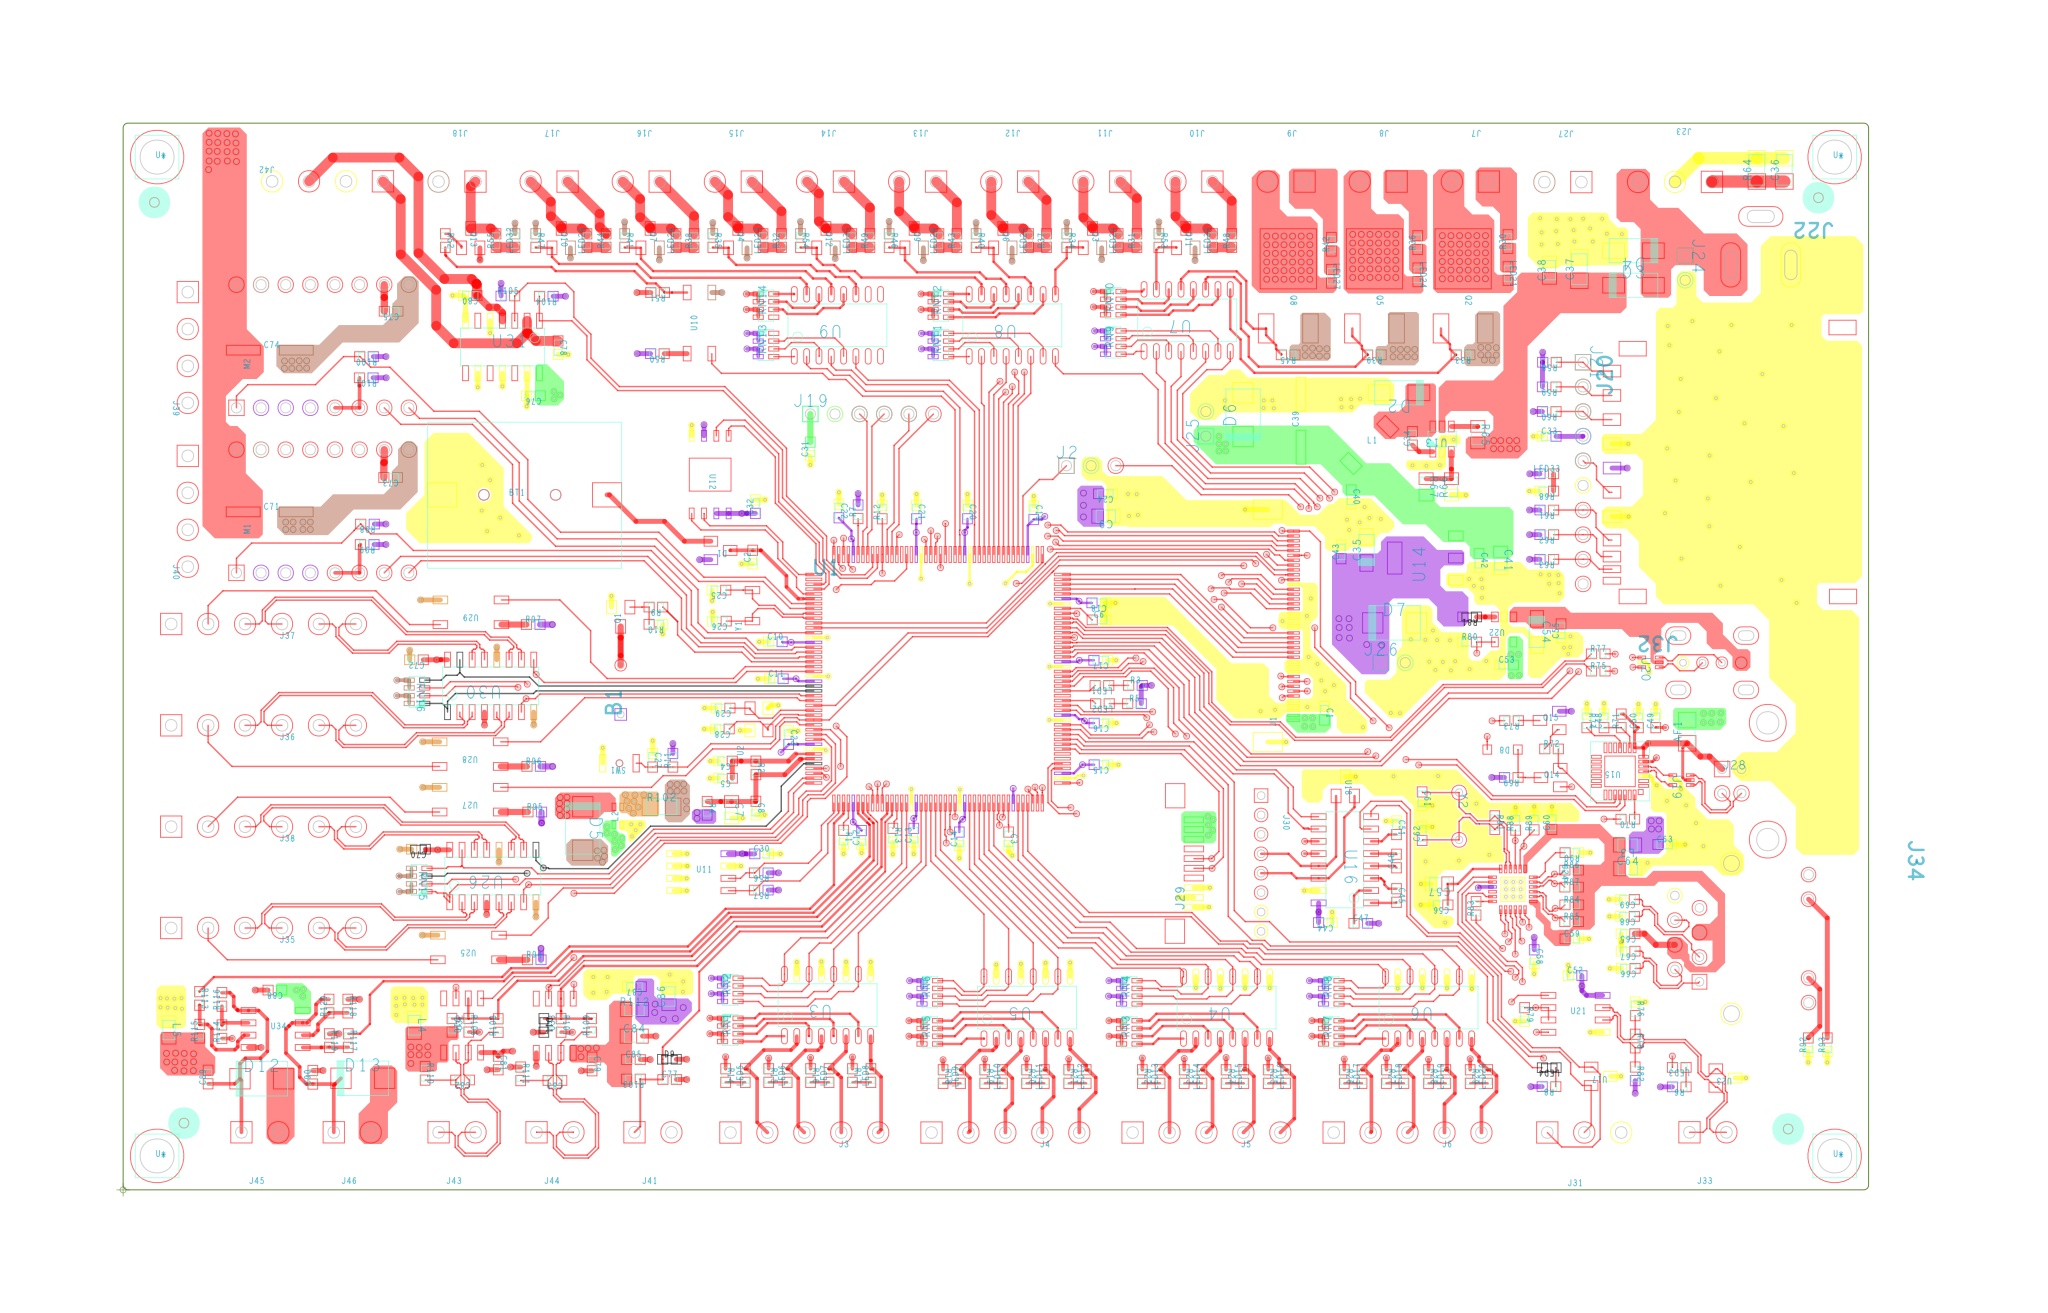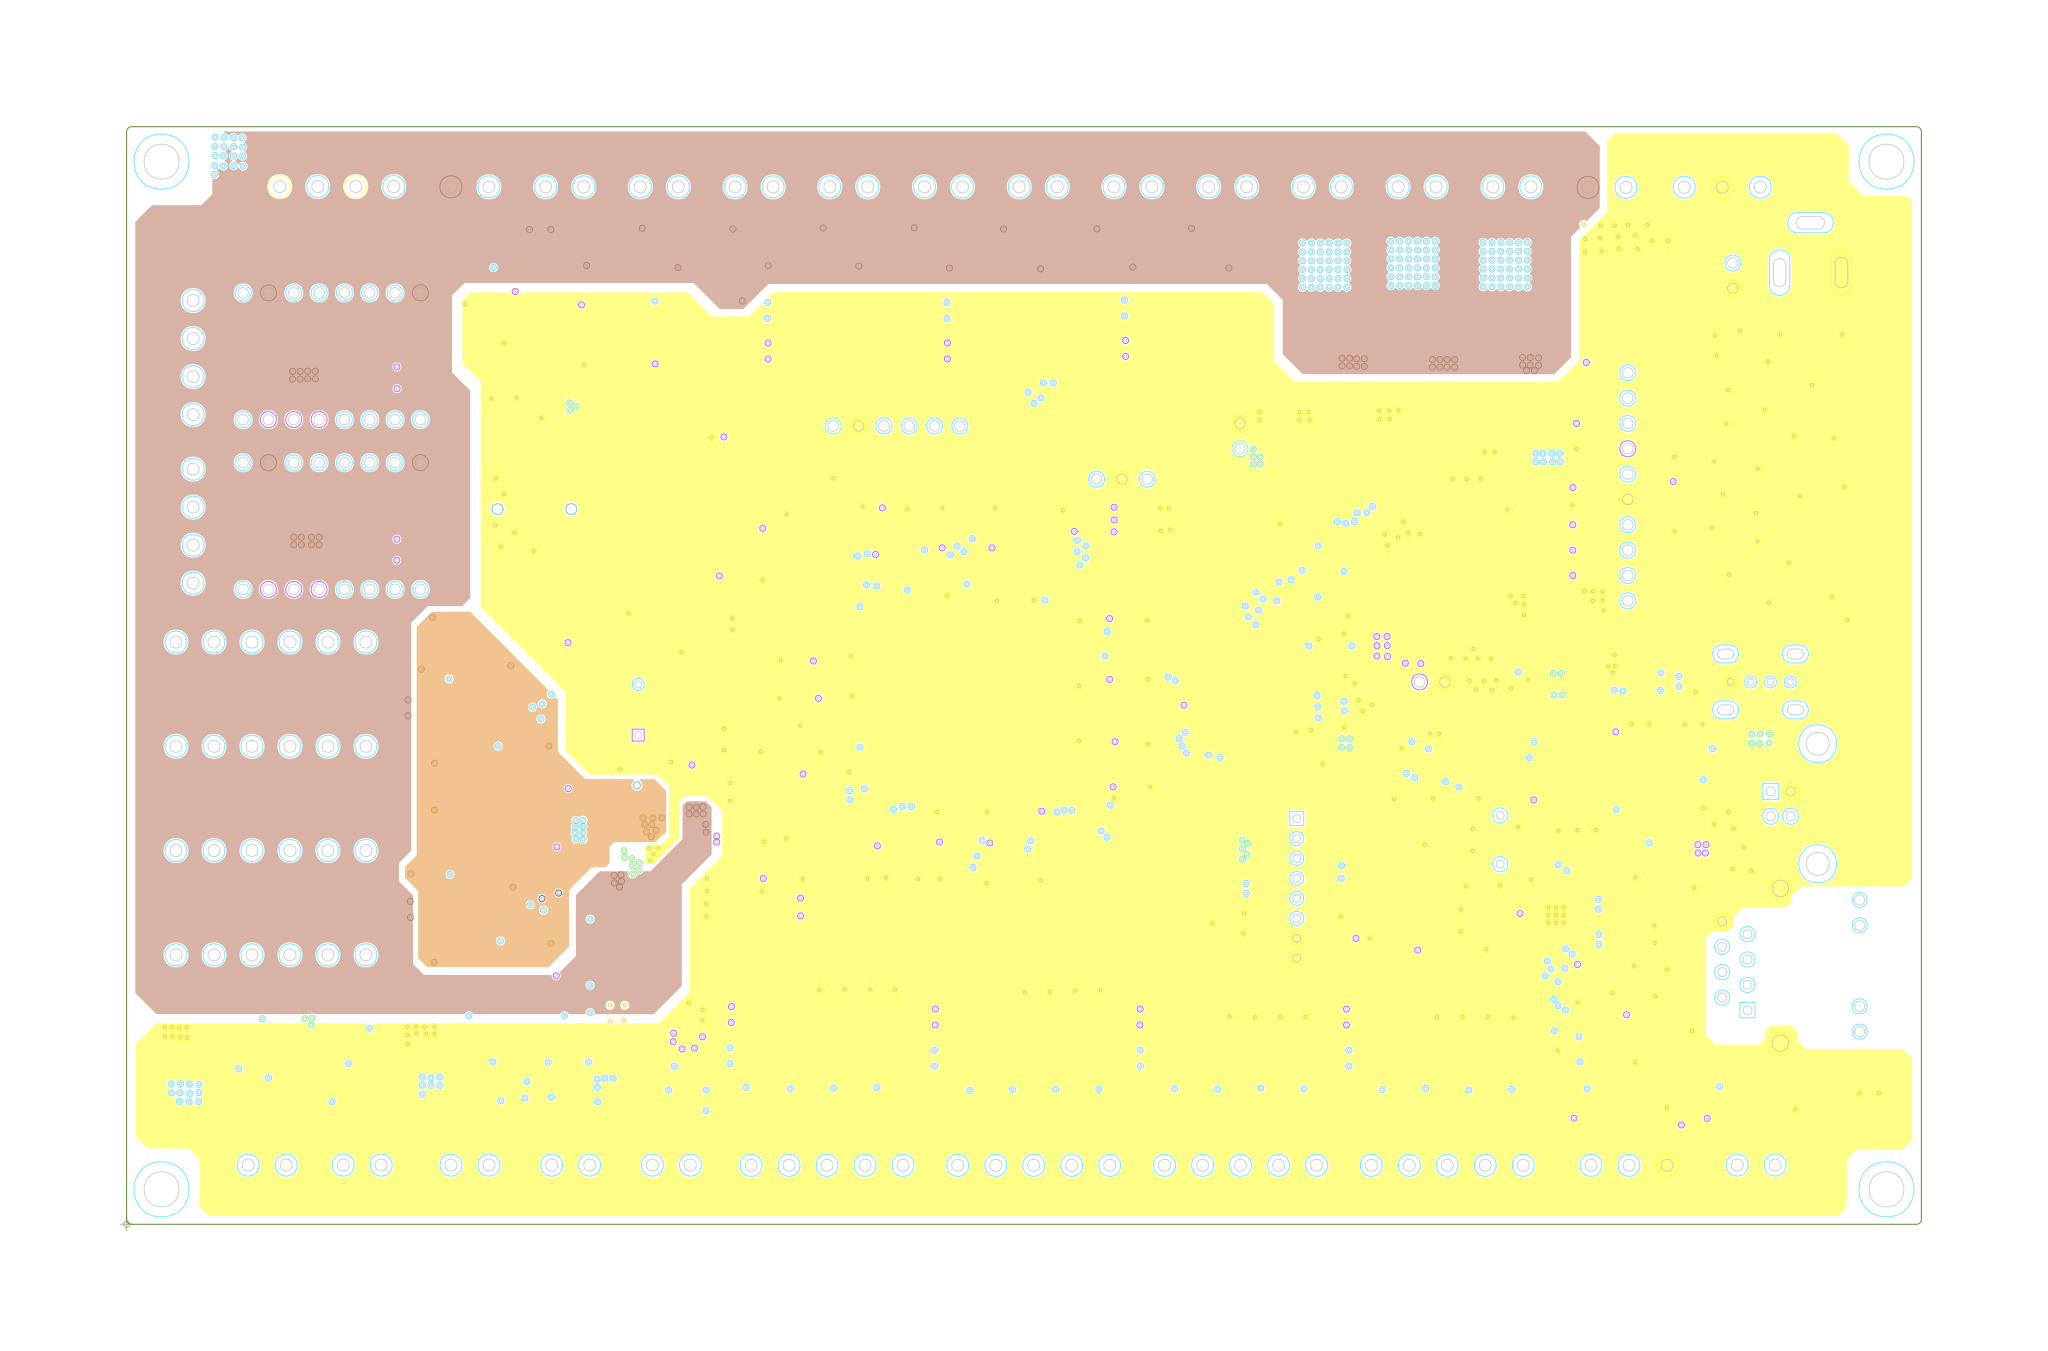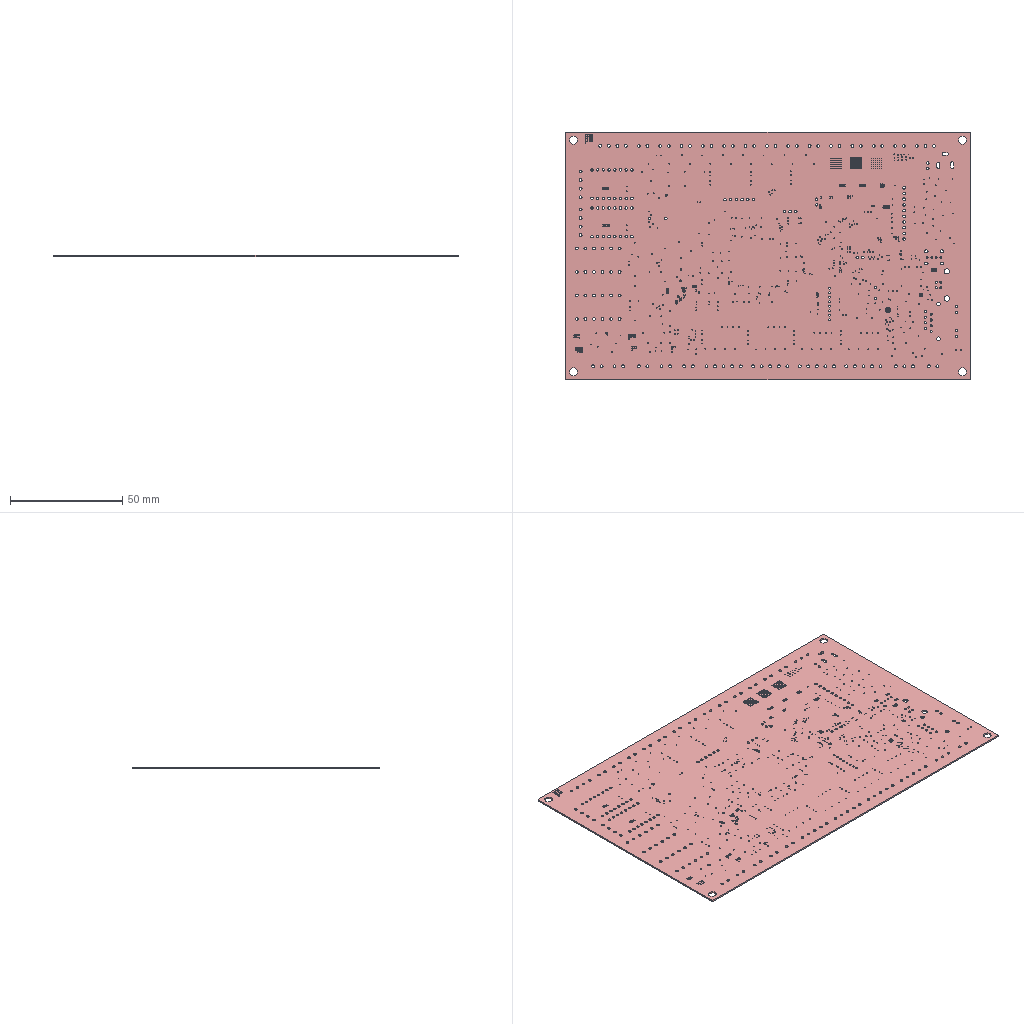Circuit board layout | Cadence Allegro | box 180 x 110 x 0.7 mm
Layer stack:
# Cadence Allegro layer stack of  (unit mm; from the constraint file cross-section; dielectric type: 0 not recorded (Allegro does not mark core vs prepreg), 3 surface material)
index,name,kind,layer,copper_thickness_mm,dielectric_type,dielectric_thickness_mm,dielectric_material,dielectric_constant
0,Top Surface,other,,,,,,
1,TOP,copper,TOP,0.0305,,,,
2,Dielectric1,dielectric,,,0,0.2032,FR-4,4.5
3,GND02,copper,GND02,0.0305,,,,
4,Dielectric2,dielectric,,,0,0.2032,FR-4,4.5
5,PWR03,copper,PWR03,0.0305,,,,
6,Dielectric3,dielectric,,,0,0.2032,FR-4,4.5
7,BOTTOM,copper,BOTTOM,0.0305,,,,
8,Bottom Surface,other,,,,,,
# drill layer pairs: low layer,high layer
drill_pair,TOP,BOTTOM
Part placement:
REFDES,COMP_VALUE,SYM_NAME,SYM_X,SYM_Y,SYM_ROTATE,SYM_MIRROR
AF1,500mA,R1206,6350.000,1860.000,90.000,NO
B1,BEEP,BELL-5,2020.000,1930.000,90.000,NO
BT1,BATTERY,BATSO,2004.016,2821.579,0.000,NO
C1,0.1uF,C0603,4877.402,1935.000,270.000,NO
C2,0.1uF,C0603,2556.000,2569.000,90.000,NO
C3,2.2uF,C0603,3595.000,1425.000,270.000,NO
C4,0.1uF,C0603,2445.701,1741.000,180.000,NO
C5,2.2uF,C0603,2445.701,1671.000,180.000,NO
C6,2.2uF,C0603,3962.000,2314.000,0.000,NO
C7,10uF,C0805,2470.000,1543.000,270.000,NO
C8,0.1uF,C0603,2569.000,1550.000,270.000,NO
C9,10uF,C0805,3990.000,2735.000,180.000,NO
C10,0.1uF,C0603,2648.000,2225.000,0.000,NO
C11,0.1uF,C0603,2652.000,2075.000,0.000,NO
C12,0.1uF,C0603,2998.000,1431.000,90.000,NO
C13,0.1uF,C0603,3210.000,1440.000,90.000,NO
C14,0.1uF,C0603,3395.000,1425.000,90.000,NO
C15,0.1uF,C0603,3970.000,1726.000,180.000,NO
C16,0.1uF,C0603,3970.000,1895.000,180.000,NO
C17,0.1uF,C0603,3969.000,2150.000,180.000,NO
C18,0.1uF,C0603,3961.000,2383.000,180.000,NO
C19,0.1uF,C0603,3697.000,2749.000,270.000,NO
C20,0.1uF,C0603,3428.000,2752.000,270.000,NO
C21,0.1uF,C0603,3221.000,2752.000,270.000,NO
C22,0.1uF,C0603,2906.000,2756.000,270.000,NO
C23,0.1uF,C0603,2702.000,1836.000,270.000,NO
C24,0.1uF,C0603,3988.000,2826.000,180.000,NO
C25,6pF,C0603,2419.000,2435.000,180.000,NO
C26,6pF,C0603,2421.000,2309.000,180.000,NO
C27,0.1uF,C0603,2150.000,1744.000,270.000,NO
C28,22pF,C0603,2433.000,1871.000,180.000,NO
C29,22pF,C0603,2436.000,1956.000,180.000,NO
C30,0.1uF,C0603,2592.000,1364.000,0.000,NO
C31,0.1uF,C0603,2790.000,3008.000,90.000,NO
C32,0.1uF,C0603,2567.000,2774.000,90.000,NO
C33,0.1uF,C0603,5790.000,3059.000,0.000,NO
C34,0.01uF,C0603,5235.000,3051.000,90.000,NO
C35,10V/10uF,TA3216,5048.000,2598.000,90.000,NO
C36,1nF/250V,C1206,6745.000,4141.000,90.000,NO
C37,10uF 50V,C1206,5912.406,3738.000,90.000,NO
C38,0.1uF 50V,C0805,5791.000,3734.000,90.000,NO
C39,16V/220uF,SMD-EC-6_3,4782.000,3015.000,90.000,NO
C40,0.1uF,C0603,4986.000,2814.000,270.000,NO
C41,10uF,C0805,5593.000,2556.000,270.000,NO
C42,0.1uF,C0603,5505.000,2556.000,270.000,NO
C43,0.1uF,C0603,4945.000,2590.000,90.000,NO
C44,0.1uF,C0603,4881.000,1085.000,180.000,NO
C45,0.1uF,C0603,5170.000,1195.000,270.000,NO
C46,0.1uF,C0603,5170.000,1335.000,90.000,NO
C47,0.1uF,C0603,5025.000,1082.000,0.000,NO
C48,0.1uF,C0603,6012.402,1904.055,90.000,NO
C49,0.1uF,C0603,6222.406,1904.055,90.000,NO
C50,0.1uF,C0603,6152.402,1904.055,90.000,NO
C51,0.1uF,C0603,5170.000,1470.000,270.000,NO
C52,0.1uF,C0603,5895.000,870.000,0.000,NO
C53,0.1uF,C0603,5617.000,2131.000,0.000,NO
C54,22uF,TA3216,5740.000,2265.000,270.000,NO
C55,0.1uF,C0603,5838.000,2270.000,90.000,NO
C56,0.1uF,C0603,5351.000,1157.000,180.000,NO
C57,10uF,C0805,5344.000,1242.000,180.000,NO
C58,0.1uF,C0603,5729.000,947.000,270.000,NO
C59,0.1uF,C0603,5882.000,1019.000,0.000,NO
C60,0.1uF,C0603,5801.000,1491.000,90.000,NO
C61,22pF,C0603,5274.000,1588.000,270.000,NO
C62,22pF,C0603,5274.000,1446.000,90.000,NO
C63,0.1uF,C0603,6259.000,1402.000,0.000,NO
C64,10uF,C0805,6109.000,1304.000,0.000,NO
C65,22nF,C0603,6110.000,1040.000,180.000,NO
C66,10pF,C0603,6111.000,899.000,180.000,NO
C67,10pF,C0603,6110.402,969.000,180.000,NO
C68,10pF,C0603,6108.000,1110.000,180.000,NO
C69,10pF,C0603,6108.000,1179.000,180.000,NO
C70,0.1uF,C0603,1199.000,1383.000,180.000,NO
C71,100uF 35V,SMD-EC-6_3,487.500,2752.500,0.000,NO
C72,0.1uF,C0603,1191.000,2152.000,180.000,NO
C73,0.1uF,C0603,1086.000,2892.000,180.000,NO
C74,100uF 35V,SMD-EC-6_3,488.000,3409.000,0.000,NO
C75,0.1uF,C0603,1088.000,3567.000,180.000,NO
C76,0.1uF,C0603,1666.000,3224.000,180.000,NO
C77,0.1uF,C0603,2219.000,448.000,0.000,NO
C78,0.1uF,C0603,1766.000,3419.000,270.000,NO
C79,0.1uF,C0603,1904.000,511.000,270.000,NO
C80,0.1uF,C0603,1409.000,3631.000,180.000,NO
C81,0.1uF,C0603,1523.000,515.000,270.000,NO
C82,0.1uF,C0603,1378.000,446.000,180.000,NO
C83,0.1uF,C0603,1753.000,444.000,180.000,NO
C84,10uF,C0805,2075.000,624.000,0.000,NO
C85,0.1uF,C0603,2072.000,529.000,0.000,NO
C86,10uF,C0805,2216.000,785.000,90.000,NO
C87,0.1uF,C0603,2076.000,825.000,180.000,NO
C88,0.1uF,C0603,616.000,811.000,180.000,NO
C89,0.1uF,C0603,345.000,458.000,90.000,NO
C90,0.1uF,C0603,770.000,457.000,90.000,NO
D1,BAT54C,SOT-23,2425.000,2596.000,180.000,NO
D2,SS14,DO-214AC,5180.000,3236.000,180.000,NO
D3,SS14,DO-214AC,6132.110,3672.409,0.000,NO
D4,SS14,DO-214AC,6132.000,3813.000,180.000,NO
D5,SMBJ5.0A,DO-214AA,1866.000,1467.000,270.000,NO
D6,SMBJ5.0A,DO-214AA,4547.000,3147.000,90.000,NO
D7,SMBJ3.3A,DO-214AA,5162.000,2301.803,0.000,NO
D8,1N4148,SOD123,5662.445,1787.402,180.000,NO
D9,CG0603MLC,R0603,2218.000,530.000,0.000,NO
D10,CG0603MLC,R0603,1335.071,668.051,270.000,NO
D11,CG0603MLC,R0603,1708.000,667.433,270.000,NO
D12,SMBJ10CA,DO-214AA,563.000,451.000,0.000,NO
D13,SMBJ10CA,DO-214AA,973.000,453.000,0.000,NO
J1,RGBLCD,FPC-TOP40,4755.890,1906.642,90.000,NO
J2,SWD,CON2_54X1X3,3830.000,2940.000,0.000,NO
J3,HEADER 5,SIP3_81X1X5,2465.591,232.638,0.000,NO
J4,HEADER 5,SIP3_81X1X5,3281.969,232.638,0.000,NO
J5,HEADER 5,SIP3_81X1X5,4098.346,232.638,0.000,NO
J6,HEADER 5,SIP3_81X1X5,4914.724,232.638,0.000,NO
J7,HEADER 2,SIP3_81X1X2,5544.626,4093.402,180.000,NO
J8,HEADER 2,SIP3_81X1X2,5170.610,4093.402,180.000,NO
J9,HEADER 2,SIP3_81X1X2,4796.594,4093.402,180.000,NO
J10,HEADER 2,SIP3_81X1X2,4422.579,4093.402,180.000,NO
J11,HEADER 2,SIP3_81X1X2,4048.563,4093.402,180.000,NO
J12,HEADER 2,SIP3_81X1X2,3674.547,4093.402,180.000,NO
J13,HEADER 2,SIP3_81X1X2,3300.531,4093.402,180.000,NO
J14,HEADER 2,SIP3_81X1X2,2926.516,4093.402,180.000,NO
J15,HEADER 2,SIP3_81X1X2,2552.500,4093.402,180.000,NO
J16,HEADER 2,SIP3_81X1X2,2178.484,4093.402,180.000,NO
J17,HEADER 2,SIP3_81X1X2,1804.469,4093.402,180.000,NO
J18,HEADER 2,SIP3_81X1X2,1430.453,4093.402,180.000,NO
J19,ATK MODULE,CON2_54X1X6,2790.000,3150.000,0.000,NO
J20,SD_CARD_L,SDCARD_L,6044.500,3225.000,90.000,NO
J21,SD,CON2_54X1X10,5927.402,3360.000,270.000,NO
J22,DC_SOCKET,DC10B,6946.000,3925.130,180.000,NO
J23,SIP3-3.81,SIP3_81X1X3,6450.551,4092.165,180.000,NO
J24,TEST24V,CON2_54X1X2,6342.000,3793.000,270.000,NO
J25,TEST5V,CON2_54X1X2,4396.000,3060.000,90.000,NO
J26,TEST3.3V,CON2_54X1X2,5105.469,2140.000,0.000,NO
J27,HEADER 2,SIP3_81X1X2,5920.354,4091.378,180.000,NO
J28,USB_TYPEB,USB-B-90,6491.846,1708.260,0.000,NO
J29,TTL_LCD,FFC-1_0-10P,4307.827,1136.035,90.000,NO
J30,UART_LCD,CI0608,4620.157,1600.591,270.000,NO
J31,RS232,SIP3_81X1X3,5782.126,232.835,0.000,NO
J32,USB-A-90,USB-A-90,6313.701,2246.303,180.000,NO
J33,HEADER 2,SIP3_81X1X2,6359.370,233.622,0.000,NO
J34,RJ45,HR911105A,6650.000,1020.004,270.000,NO
J35,X  AXIS,SIP3_81X1X6,195.000,1063.071,0.000,NO
J36,Z  AXIS,SIP3_81X1X6,195.000,1885.906,0.000,NO
J37,A  AXIS,SIP3_81X1X6,195.000,2297.323,0.000,NO
J38,Y AXIS,SIP3_81X1X6,195.000,1474.488,0.000,NO
J39,C  AXIS,SIP3_81X1X4,262.441,3644.803,270.000,NO
J40,B  AXIS,SIP3_81X1X4,262.441,2979.803,270.000,NO
J41,HEADER 2,SIP3_81X1X2,2076.063,233.622,0.000,NO
J42,HEADER 4,SIP3_81X1X4,1054.803,4094.583,180.000,NO
J43,HEADER 2,SIP3_81X1X2,1280.787,233.622,0.000,NO
J44,HEADER 2,SIP3_81X1X2,1678.425,233.622,0.000,NO
J45,HEADER 2,SIP3_81X1X2,480.197,233.622,0.000,NO
J46,HEADER 2,SIP3_81X1X2,855.197,233.622,0.000,NO
L1,4.7uH,SMD-L5_1W5_1_H3_0,5060.000,3024.000,0.000,NO
L2,ACM2012,ACM2012,1993.000,1482.000,90.000,NO
L3,220R,2A,0.05DCR,R0805,6108.000,1400.000,180.000,NO
L4,330OHM,R0805,1182.000,668.000,270.000,NO
L5,330OHM,R0805,186.000,649.000,270.000,NO
LED1,LED,LED0603,3974.000,2048.000,180.000,NO
LED2,LED,LED0603,3976.000,1974.000,180.000,NO
LED3,LED,LED0603,6318.000,497.000,180.000,NO
LED4,LED,LED0603,5790.000,496.000,180.000,NO
LED5,LED,LED0603,2526.000,464.000,90.000,NO
LED6,LED,LED0603,2696.000,464.000,90.000,NO
LED7,LED,LED0603,2866.000,464.000,90.000,NO
LED8,LED,LED0603,3036.000,464.000,90.000,NO
LED9,LED,LED0603,3400.000,460.000,90.000,NO
LED10,LED,LED0603,3570.000,460.000,90.000,NO
LED11,LED,LED0603,3740.000,460.000,90.000,NO
LED12,LED,LED0603,3910.000,460.000,90.000,NO
LED13,LED,LED0603,4210.000,460.000,90.000,NO
LED14,LED,LED0603,4380.000,460.000,90.000,NO
LED15,LED,LED0603,4550.000,460.000,90.000,NO
LED16,LED,LED0603,4720.000,460.000,90.000,NO
LED17,LED,LED0603,5030.000,460.000,90.000,NO
LED18,LED,LED0603,5200.000,460.000,90.000,NO
LED19,LED,LED0603,5370.000,460.000,90.000,NO
LED20,LED,LED0603,5540.000,460.000,90.000,NO
LED21,LED,LED0603,5622.551,3720.000,270.000,NO
LED22,LED,LED0603,4040.055,3854.000,90.000,NO
LED23,LED,LED0603,2598.055,3854.000,90.000,NO
LED24,LED,LED0603,5256.551,3715.000,270.000,NO
LED25,LED,LED0603,3676.055,3854.000,90.000,NO
LED26,LED,LED0603,2245.055,3854.000,90.000,NO
LED27,LED,LED0603,4905.551,3709.000,270.000,NO
LED28,LED,LED0603,3312.055,3854.000,90.000,NO
LED29,LED,LED0603,1883.055,3854.000,90.000,NO
LED30,LED,LED0603,4423.000,3854.000,90.000,NO
LED31,LED,LED0603,2958.055,3854.000,90.000,NO
LED32,LED,LED0603,1591.000,3854.000,90.000,NO
LED33,LED,LED0603,5780.000,2907.000,0.000,NO
M1,STEPSTICK,STEPSTICK,460.000,2505.000,90.000,NO
M2,STEPSTICK,STEPSTICK,460.000,3175.000,90.000,NO
Q1,8050,SOT-23,2020.000,2327.000,90.000,NO
Q2,FR540,TO-252AA,5440.551,3780.000,270.000,NO
Q3,PMV60EN,SOT-23,3935.528,3863.500,270.000,NO
Q4,PMV60EN,SOT-23,2495.528,3863.500,270.000,NO
Q5,FR540,TO-252AA,5080.551,3780.000,270.000,NO
Q6,PMV60EN,SOT-23,3571.528,3863.500,270.000,NO
Q7,PMV60EN,SOT-23,2139.528,3863.500,270.000,NO
Q8,FR540,TO-252AA,4730.551,3780.000,270.000,NO
Q9,PMV60EN,SOT-23,3211.528,3863.500,270.000,NO
Q10,PMV60EN,SOT-23,1778.528,3863.500,270.000,NO
Q11,PMV60EN,SOT-23,4314.528,3863.500,270.000,NO
Q12,PMV60EN,SOT-23,2853.528,3863.500,270.000,NO
Q13,PMV50EP,SOT-23,1411.000,3863.500,270.000,NO
Q14,S8050,SOT-23,5795.902,1673.555,0.000,NO
Q15,S8550,SOT-23,5791.902,1905.555,0.000,NO
R1,10K,R0603,2925.000,1432.000,270.000,NO
R2,10R,R0603,2569.000,1713.000,270.000,NO
R3,510R,R0603,4110.000,2048.000,0.000,NO
R4,10R,R0603,2371.000,1549.000,270.000,NO
R5,510R,R0603,4106.000,1974.000,0.000,NO
R6,510R,R0603,6318.000,418.000,180.000,NO
R7,0R,R0603,2984.000,2753.000,90.000,NO
R8,510R,R0603,5789.000,419.000,180.000,NO
R9,510R,R0603,2163.000,2366.000,180.000,NO
R10,10K,R0603,2163.000,2296.000,180.000,NO
R11,10K,R0603,2232.000,1744.000,90.000,NO
R12,100K,R0603,3082.000,2752.000,90.000,NO
R13,100K,R0603,3125.000,1440.000,270.000,NO
R14,3.9K,R0603,2446.000,464.000,270.000,NO
R15,3.9K,R0603,2621.000,464.000,270.000,NO
R16,3.9K,R0603,2791.000,464.000,270.000,NO
R17,3.9K,R0603,2961.000,464.000,270.000,NO
R18,3.9K,R0603,3329.000,460.000,270.000,NO
R19,3.9K,R0603,3498.000,460.000,270.000,NO
R20,3.9K,R0603,3668.000,460.000,270.000,NO
R21,3.9K,R0603,3839.000,460.000,270.000,NO
R22,3.9K,R0603,4138.000,460.000,270.000,NO
R23,3.9K,R0603,4308.000,460.000,270.000,NO
R24,3.9K,R0603,4478.000,460.000,270.000,NO
R25,3.9K,R0603,4649.000,460.000,270.000,NO
R26,3.9K,R0603,4958.000,460.000,270.000,NO
R27,3.9K,R0603,5129.000,460.000,270.000,NO
R28,3.9K,R0603,5300.000,460.000,270.000,NO
R29,3.9K,R0603,5469.000,460.000,270.000,NO
R30,4.7K,R0603,5622.551,3850.000,90.000,NO
R31,4.7K,R0603,4116.000,3854.000,90.000,NO
R32,4.7K,R0603,2673.000,3854.000,90.000,NO
R33,100K,R0603,5440.000,3390.000,180.000,NO
R34,100K,R0603,3831.000,3854.000,270.000,NO
R35,100K,R0603,2394.000,3854.000,270.000,NO
R36,4.7K,R0603,5256.000,3846.000,90.000,NO
R37,4.7K,R0603,3749.000,3854.000,90.000,NO
R38,4.7K,R0603,2318.000,3854.000,90.000,NO
R39,100K,R0603,5080.000,3390.000,180.000,NO
R40,100K,R0603,3463.000,3854.000,270.000,NO
R41,100K,R0603,2036.000,3854.000,270.000,NO
R42,4.7K,R0603,4905.551,3839.000,90.000,NO
R43,4.7K,R0603,3385.000,3854.000,90.000,NO
R44,4.7K,R0603,1961.000,3854.000,90.000,NO
R45,100K,R0603,4730.000,3390.000,180.000,NO
R46,100K,R0603,3110.000,3854.000,270.000,NO
R47,100K,R0603,1675.000,3854.000,270.000,NO
R48,4.7K,R0603,4501.000,3854.000,90.000,NO
R49,4.7K,R0603,3032.000,3854.000,90.000,NO
R50,1K,R0603,2169.000,3395.000,180.000,NO
R51,10K,R0603,2170.000,3643.000,180.000,NO
R52,1K,R0603,1308.000,3854.000,270.000,NO
R53,100K,R0603,4205.000,3854.000,270.000,NO
R54,100K,R0603,2750.000,3854.000,270.000,NO
R55,4.7K,R0603,1514.000,3854.000,90.000,NO
R56,4.7K,R0603,2591.000,1287.000,180.000,NO
R57,4.7K,R0603,2591.000,1217.000,180.000,NO
R58,47K,R0603,5791.000,3360.000,180.000,NO
R59,47K,R0603,5790.000,3260.000,180.000,NO
R60,47K,R0603,5790.000,3160.000,180.000,NO
R61,47K,R0603,5780.000,2760.000,180.000,NO
R62,47K,R0603,5780.000,2660.000,180.000,NO
R63,47K,R0603,5780.000,2560.000,180.000,NO
R64,1M,R1206,6633.000,4141.000,90.000,NO
R65,100K,R0805,5500.000,3066.000,270.000,NO
R66,9.53K 1%,R0805,5393.000,2854.000,90.000,NO
R67,49.9K 1%,R0805,5290.000,2854.000,270.000,NO
R68,680R,R0603,5780.000,2837.000,180.000,NO
R69,10K,R0603,5635.945,1674.402,180.000,NO
R70,1K,R0603,6109.000,1505.000,180.000,NO
R71,10K,R0603,6082.402,1904.055,90.000,NO
R72,1K,R0603,5799.402,1790.055,0.000,NO
R73,1K,R0603,5637.000,1905.000,180.000,NO
R74,10K,R0603,5942.402,1904.055,270.000,NO
R75,22R,R0603,5989.000,2106.000,0.000,NO
R76,560R,R0603,6139.000,735.000,270.000,NO
R77,22R,R0603,5989.000,2176.000,0.000,NO
R78,120R,R0603,6139.000,604.000,270.000,NO
R79,10K,R0603,5690.000,712.000,270.000,NO
R80,10K,R0603,5467.000,2224.000,0.000,NO
R81,100K,R0603,5467.000,2326.000,180.000,NO
R82,560R,R0603,6139.000,471.000,270.000,NO
R83,510R,R0603,5493.000,1143.000,90.000,NO
R84,49.9R,R0603,5881.402,1157.000,0.000,NO
R85,49.9R,R0603,5881.000,1089.000,0.000,NO
R86,49.9R,R0603,5881.000,1298.000,0.000,NO
R87,49.9R,R0603,5881.000,1229.000,0.000,NO
R88,10K,R0603,5653.402,1488.000,90.000,NO
R89,10K,R0603,5729.000,1489.000,90.000,NO
R90,12.1K,R0603,5882.000,1369.000,180.000,NO
R91,1M,R0603,5569.000,1491.000,270.000,NO
R92,510R,R0603,6842.000,589.000,90.000,NO
R93,510R,R0603,6919.000,589.000,90.000,NO
R94,1K,R0603,1669.000,934.000,0.000,NO
R95,1K,R0603,1671.000,1534.000,0.000,NO
R96,1K,R0603,1667.000,1719.000,0.000,NO
R97,1K,R0603,1665.000,2295.000,0.000,NO
R98,10K,R0603,992.000,2703.000,180.000,NO
R99,10K,R0603,991.000,2620.000,180.000,NO
R100,10K,R0603,988.000,3383.000,180.000,NO
R101,10K,R0603,987.000,3297.000,180.000,NO
R102,0R,R1206,2186.000,1555.000,0.000,NO
R103,4.7K 1%,R0603,2072.000,450.000,180.000,NO
R104,10K,R0603,1718.000,3628.000,180.000,NO
R105,10K,R0603,1562.000,3629.000,0.000,NO
R106,4.7K 1%,R0603,1403.142,668.047,270.000,NO
R107,4.7K 1%,R0603,1778.102,667.433,270.000,NO
R108,0R,R0603,1523.000,667.000,90.000,NO
R109,0R,R0603,1902.000,668.000,90.000,NO
R110,0R,R0603,1226.000,473.000,270.000,NO
R111,0R,R0603,1614.000,471.000,270.000,NO
R112,10R,R0805,2076.000,732.000,0.000,NO
R113,10K 1%,R0603,310.000,777.000,270.000,NO
R114,10K 1%,R0603,401.000,642.000,90.000,NO
R115,30K 1%,R0603,311.000,644.000,90.000,NO
R116,30K 1%,R0603,401.000,773.000,90.000,NO
R117,10K 1%,R0603,914.000,606.000,270.000,NO
R118,10K 1%,R0603,912.000,746.000,270.000,NO
R119,30K 1%,R0603,837.000,606.000,270.000,NO
R120,30K 1%,R0603,836.000,746.000,90.000,NO
RN1,3.9K,R0603X4,2464.992,649.480,0.000,NO
RN2,4.7K,R0603X4,2464.992,812.024,0.000,NO
RN3,3.9K,R0603X4,4084.992,639.480,0.000,NO
RN4,4.7K,R0603X4,4084.992,802.024,0.000,NO
RN5,3.9K,R0603X4,3274.992,639.480,0.000,NO
RN6,4.7K,R0603X4,3274.992,802.024,0.000,NO
RN7,3.9K,R0603X4,4904.992,639.480,0.000,NO
RN8,4.7K,R0603X4,4904.992,802.024,0.000,NO
RN9,1K,R0603X4,4020.000,3440.000,0.000,NO
RN10,5.1K,R0603X4,4020.000,3600.000,0.000,NO
RN11,1K,R0603X4,3320.000,3430.000,0.000,NO
RN12,5.1K,R0603X4,3320.000,3590.000,0.000,NO
RN13,1K,R0603X4,2610.000,3430.000,0.000,NO
RN14,5.1K,R0603X4,2610.000,3590.000,0.000,NO
RN15,10K,R0603X4,1202.000,1258.000,180.000,NO
RN16,10K,R0603X4,1193.000,2022.000,180.000,NO
SW1,KEY,KEY,2015.000,1732.000,180.000,NO
U1,STM32F429IGT6,LQFP176,2804.157,2498.228,0.000,NO
U2,25MHz,XTAL3225,2618.000,1865.000,90.000,NO
U3,PS2801-4,PS2805,2860.000,750.000,90.000,NO
U4,PS2801-4,PS2805,4480.000,740.000,90.000,NO
U5,PS2801-4,PS2805,3670.000,740.000,90.000,NO
U6,PS2801-4,PS2805,5300.000,740.000,90.000,NO
U7,PS2801-4,PS2805,4320.000,3530.000,90.000,NO
U8,PS2801-4,PS2805,3610.000,3510.000,90.000,NO
U9,PS2801-4,PS2805,2900.000,3510.000,90.000,NO
U10,PC357,PC357,2290.000,3395.000,90.000,NO
U11,24LC32,SO8,2237.228,1364.614,0.000,NO
U12,W25Q256,MLP8,2383.346,2903.654,270.000,NO
U13,MP2359,SOT23-6,5355.000,3048.000,90.000,NO
U14,LT1117-3.3,SOT-223,5410.500,2475.000,90.000,NO
U15,CP2102GMR,QFN-28,6077.402,1699.055,180.000,NO
U16,MAX3232,SO16,4960.000,1340.000,180.000,NO
U17,ESDA14V2L,SOT-23,5999.000,461.000,180.000,NO
U18,ESDA14V2L,SOT-23,4962.000,1638.000,270.000,NO
U19,USBLC6-2P6,SOT-666,6291.567,1683.193,270.000,NO
U20,USBLC6-2P6,SOT-666,6165.567,2161.193,270.000,NO
U21,MAX3485,SO8,5786.811,789.567,0.000,NO
U22,TPS2051BDBV,SOT-23-5,5607.000,2275.000,180.000,NO
U23,SM712,SOT-23,6505.000,454.000,180.000,NO
U24,LAN8720A,QFN24,5642.484,1220.000,270.000,NO
U25,PC357,PC357,1526.000,934.000,180.000,NO
U26,AM26C31,SO16,1501.000,1274.000,90.000,NO
U27,PC357,PC357,1533.000,1534.000,180.000,NO
U28,PC357,PC357,1533.000,1719.000,180.000,NO
U29,PC357,PC357,1536.000,2295.000,180.000,NO
U30,AM26C31,SO16,1492.000,2046.000,90.000,NO
U31,74ACT04,SO14,1540.000,3422.000,270.000,NO
U32,MAX6675,SO8,1301.386,557.244,90.000,NO
U33,MAX6675,SO8,1677.386,556.228,90.000,NO
U34,AD8606,SO8,509.000,728.000,0.000,NO
Y1,32.768KHz,XTAL3215,2555.000,2309.000,90.000,NO
Y2,25MHz,XTL_8M,5424.000,1613.000,270.000,NO
Pad and via stacks:
# Allegro (Cadence) via spans and padstacks; design units: ("mils" 3 1000)
# via spans: padstack,start_layer,end_layer,net_example,count
VIA12_24,ETCH/TOP,ETCH/BOTTOM,DAGND,851
# Allegro padstack definitions: name,start_layer,end_layer,drill,plating,holeType,type
VIA30D16,"ETCH/TOP","ETCH/BOTTOM",16.0,"PLATED","circle_drill","through"
R180_160,"ETCH/TOP","ETCH/TOP",0.0,"PLATED","none","smd"
PTH_C472D276S40,"ETCH/TOP","ETCH/BOTTOM",27.559,"PLATED","circle_drill","through"
PTH_S472D276S40,"ETCH/TOP","ETCH/BOTTOM",27.559,"PLATED","circle_drill","through"
RE118_11X98_43,"ETCH/TOP","ETCH/TOP",0.0,"NON_PLATED","none","smd"
C43_31D43_31,"ETCH/TOP","ETCH/BOTTOM",43.311,"PLATED","circle_drill","through"
R105_100,"ETCH/TOP","ETCH/TOP",0.0,"PLATED","none","smd"
R170_135,"ETCH/TOP","ETCH/TOP",0.0,"PLATED","none","smd"
R145_120,"ETCH/TOP","ETCH/TOP",0.0,"PLATED","none","smd"
RE350X100,"ETCH/TOP","ETCH/TOP",0.0,"PLATED","none","smd"
RE55X40,"ETCH/TOP","ETCH/TOP",0.0,"NON_PLATED","none","smd"
R225_160,"ETCH/TOP","ETCH/TOP",0.0,"PLATED","none","smd"
S210,"ETCH/TOP","ETCH/TOP",0.0,"PLATED","none","smd"
RE90X95,"ETCH/TOP","ETCH/TOP",0.0,"NON_PLATED","none","smd"
SMD_R787X1181P0S40,"ETCH/TOP","ETCH/TOP",0.0,"PLATED","none","smd"
SMD_R98X472P0S40,"ETCH/TOP","ETCH/TOP",0.0,"PLATED","none","smd"
S220H120T220_240_40,"ETCH/TOP","ETCH/BOTTOM",47.244,"PLATED","circle_drill","through"
C220H120T220_240_40,"ETCH/TOP","ETCH/BOTTOM",47.244,"PLATED","circle_drill","through"
S160H105T155_190_40,"ETCH/TOP","ETCH/BOTTOM",41.339,"PLATED","circle_drill","through"
C160H105T155_190_40,"ETCH/TOP","ETCH/BOTTOM",41.339,"PLATED","circle_drill","through"
SMD_R472X709P0S40,"ETCH/TOP","ETCH/TOP",0.0,"PLATED","none","smd"
SMD_R276X709P0S40,"ETCH/TOP","ETCH/TOP",0.0,"PLATED","none","smd"
SMD_R591X1102P0S40,"ETCH/TOP","ETCH/TOP",0.0,"PLATED","none","smd"
SMD_R433X709P0S40,"ETCH/TOP","ETCH/TOP",0.0,"PLATED","none","smd"
PTH_O1800X800SLOT500X1100S40,"ETCH/TOP","ETCH/BOTTOM",50.0,"PLATED","oval slot","through"
PTH_O800X1800SLOT500X1200S40,"ETCH/TOP","ETCH/BOTTOM",50.0,"PLATED","oval slot","through"
PTH_O800X1800SLOT500X1100S40,"ETCH/TOP","ETCH/BOTTOM",50.0,"PLATED","oval slot","through"
PTH_S630D362S40,"ETCH/TOP","ETCH/BOTTOM",36.22,"PLATED","circle_drill","through"
PTH_C630D362S40,"ETCH/TOP","ETCH/BOTTOM",36.22,"PLATED","circle_drill","through"
PTH_C1496D906S40,"ETCH/TOP","ETCH/BOTTOM",90.551,"PLATED","circle_drill","through"
SMD_R984X787P0S40,"ETCH/TOP","ETCH/TOP",0.0,"PLATED","none","smd"
SMD_R236X787P0S40,"ETCH/TOP","ETCH/TOP",0.0,"PLATED","none","smd"
S140H80,"ETCH/TOP","ETCH/BOTTOM",31.496,"PLATED","circle_drill","through"
C140H80,"ETCH/TOP","ETCH/BOTTOM",31.496,"PLATED","circle_drill","through"
S140H90T140_170_40,"ETCH/TOP","ETCH/BOTTOM",35.433,"PLATED","circle_drill","through"
C140H90T140_170_40,"ETCH/TOP","ETCH/BOTTOM",35.433,"PLATED","circle_drill","through"
C355H235T285_330_50,"ETCH/TOP","ETCH/BOTTOM",92.52,"PLATED","circle_drill","through"
PTH_C591D402S40,"ETCH/TOP","ETCH/BOTTOM",40.161,"PLATED","circle_drill","through"
PTH_C600D350S40,"ETCH/TOP","ETCH/BOTTOM",35.0,"PLATED","circle_drill","through"
PTH_C866D650S40,"ETCH/TOP","ETCH/BOTTOM",64.961,"PLATED","circle_drill","through"
PTH_S600D350S40,"ETCH/TOP","ETCH/BOTTOM",35.0,"PLATED","circle_drill","through"
RE200X125,"ETCH/TOP","ETCH/TOP",0.0,"PLATED","none","smd"
RE75X40,"ETCH/TOP","ETCH/TOP",0.0,"NON_PLATED","none","smd"
SQ120,"ETCH/TOP","ETCH/TOP",0.0,"PLATED","none","smd"
RE620X580,"ETCH/TOP","ETCH/TOP",0.0,"NON_PLATED","none","smd"
RE300X160,"ETCH/TOP","ETCH/TOP",0.0,"NON_PLATED","none","smd"
C100H60,"ETCH/TOP","ETCH/BOTTOM",23.622,"PLATED","circle_drill","through"
RE100H60,"ETCH/TOP","ETCH/BOTTOM",23.622,"PLATED","circle_drill","through"
R105_45,"ETCH/TOP","ETCH/TOP",0.0,"PLATED","none","smd"
RE65X180,"ETCH/TOP","ETCH/TOP",0.0,"PLATED","none","smd"
H70,"ETCH/TOP","ETCH/BOTTOM",27.559,"PLATED","circle_drill","through"
SMD_R100X650P0S40,"ETCH/TOP","ETCH/TOP",0.0,"PLATED","none","smd"
RE150X80,"ETCH/TOP","ETCH/TOP",0.0,"NON_PLATED","none","smd"
SMD_R512X413P0S40,"ETCH/TOP","ETCH/TOP",0.0,"PLATED","none","smd"
RE60X24,"ETCH/TOP","ETCH/TOP",0.0,"NON_PLATED","none","smd"
RE43_31X19_68,"ETCH/TOP","ETCH/TOP",0.0,"PLATED","none","smd"
RE134X170,"ETCH/TOP","ETCH/TOP",0.0,"PLATED","none","smd"
R110_60,"ETCH/TOP","ETCH/TOP",0.0,"PLATED","none","smd"
RE100X150,"ETCH/TOP","ETCH/TOP",0.0,"PLATED","none","smd"
RE330X150,"ETCH/TOP","ETCH/TOP",0.0,"PLATED","none","smd"
RE39_37X11_81,"ETCH/TOP","ETCH/TOP",0.0,"NON_PLATED","none","smd"
RE11_81X39_37,"ETCH/TOP","ETCH/TOP",0.0,"NON_PLATED","none","smd"
SQ124,"ETCH/TOP","ETCH/TOP",0.0,"NON_PLATED","none","smd"
SQ20,"ETCH/TOP","ETCH/TOP",0.0,"NON_PLATED","none","smd"
R155_60,"ETCH/TOP","ETCH/TOP",0.0,"PLATED","none","smd"
SMD_R118X315P0S40,"ETCH/TOP","ETCH/TOP",0.0,"PLATED","none","smd"
R27X39,"ETCH/TOP","ETCH/TOP",0.0,"PLATED","none","smd"
SMD_R98X315P0S40,"ETCH/TOP","ETCH/TOP",0.0,"PLATED","none","smd"
SMD_S984P0S40,"ETCH/TOP","ETCH/TOP",0.0,"PLATED","none","smd"
SMD_R591X295P0S40,"ETCH/TOP","ETCH/TOP",0.0,"PLATED","none","smd"
SMD_R295X591P0S40,"ETCH/TOP","ETCH/TOP",0.0,"PLATED","none","smd"
PTH_C600D300S40,"ETCH/TOP","ETCH/BOTTOM",30.0,"PLATED","circle_drill","through"
C177_17D137_80,"ETCH/TOP","ETCH/BOTTOM",137.799,"PLATED","circle_drill","through"
B160_60,"ETCH/TOP","ETCH/TOP",0.0,"PLATED","none","smd"
PTH_O1024X709SLOT394X630S40,"ETCH/TOP","ETCH/BOTTOM",39.37,"PLATED","oval slot","through"
VIA12_24,"ETCH/TOP","ETCH/BOTTOM",12.0,"PLATED","circle_drill","through"
Y300,"ETCH/TOP","ETCH/BOTTOM",118.11,"NON_PLATED","circle_drill","through"
C83D53,"ETCH/TOP","ETCH/BOTTOM",53.0,"PLATED","circle_drill","through"
R18X20,"ETCH/TOP","ETCH/TOP",0.0,"NON_PLATED","none","smd"
Y3,"ETCH/TOP","ETCH/TOP",0.0,"PLATED","none","smd"
Design rules, without the lines most boards share, first 19 of 41 lines:
# Cadence Allegro design rules of  (from the Constraint Manager export constraints.dcfx, design unit mil; typed fields in mm)
# columns: name | kind | enabled | priority | scope1 | scope2 | descriptor | typed fields (field=value)
# Allegro precedence (priority 1 wins): 1 Region class-to-class, 2 Region class, 3 Region, 4 class-to-class, 5 DiffPair/Bus/NetGroup override, 6 NetClass, 7 constraint set (CSet) default
# per-layer values are written LAYER=value in the descriptor and LAYER:mm in the typed field; a maximum of 0 means no limit set
# --- net classes (and buses / net groups) ---
# (no net classes defined: every net uses the default constraint sets)
# --- track widths, neck and differential-pair gap (physical constraint sets) ---
DEFAULT | PhysicalCSet | enabled | 7 | Design default | All | Physical Constraint (Min Line Width=6mil) (Max Line Width=100mil) (Min Neck Width=6mil) (Max Neck Length=6mil) (DiffPair Primary Gap=6mil) (DiffPair Neck Gap=6mil) (DiffPair Min Space=6mil) (DiffPair Coupled +Tol=6mil) (DiffPair Coupled -Tol=6mil) (Min BB Via Stagger=6mil) (Max BB Via Stagger=6mil) (T-junctions=ANYWHERE) (Pad-pad direct connect=ALL_ALLOWED) (Allowed vias=VIA12_24) | min_line_width=0.1524 min_neck_width=0.1524 min_bvia_stagger=0.1524 max_bvia_stagger=0.1524 ts_allowed=ANYWHERE diffp_primary_gap=0.1524 diffp_neck_gap=0.1524 max_line_width=2.54 maximum_neck_length=0.1524 pad_pad_direct_connect=ALL_ALLOWED allow_on_etch_subclass=TRUE diffp_coupled_plus=0.1524 diffp_coupled_minus=0.1524 diffp_min_space=0.1524 vias=VIA12_24
# --- clearances: line / pad / via / shape / hole (spacing constraint sets) ---
DEFAULT | SpacingCSet | enabled | 7 | Design default | All | Clearance Constraint (Line-Line=6mil) (Line-SMD Pad=6mil) (Line-Thru Pin=6mil) (Line-Via=6mil) (Line-Shape=6mil) (SMD Pad-SMD Pad=7mil) (Thru Pin-Thru Pin=7mil) (Thru Pin-SMD Pad=7mil) (SMD Pad-Via=6mil) (Thru Pin-Via=6mil) (Via-Via=6mil) (Shape-SMD Pad=6mil) (Shape-Thru Pin=6mil) (Shape-Via=6mil) (Shape-Shape=6mil) (Hole-Hole=8mil) (Hole-Line=6mil) (Hole-Shape=8mil) (BB Via-BB Via=6mil) (uVia-uVia=5mil) | thrupin_to_thrupin_spacing=0.1778 thrupin_to_smdpin_spacing=0.1778 thrupin_to_thruvia_spacing=0.1524 line_to_thrupin_spacing=0.1524 thrupin_to_shape_spacing=0.1524 smdpin_to_smdpin_spacing=0.1778 smdpin_to_thruvia_spacing=0.1524 line_to_smdpin_spacing=0.1524 shape_to_smdpin_spacing=0.1524 thruvia_to_thruvia_spacing=0.1524 line_to_thruvia_spacing=0.1524 shape_to_thruvia_spacing=0.1524 line_to_line_spacing=0.1524 line_to_shape_spacing=0.1524 shape_to_shape_spacing=0.1524 bbv_to_bbv_spacing=0.1524 bbv_to_thrupin_spacing=0.1524 bbv_to_smdpin_spacing=0.1524 bbv_to_thruvia_spacing=0.1524 bbv_to_line_spacing=0.1524 bbv_to_shape_spacing=0.1524 bbv_to_testpin_spacing=0.1524 bbv_to_testvia_spacing=0.1524 testpin_to_testpin_spacing=0.1778 testpin_to_thrupin_spacing=0.1778 smdpin_to_testpin_spacing=0.1778 testpin_to_thruvia_spacing=0.1524 testpin_to_testvia_spacing=0.1524 line_to_testpin_spacing=0.1524 shape_to_testpin_spacing=0.1524 testvia_to_testvia_spacing=0.127 testvia_to_thrupin_spacing=0.1524 smdpin_to_testvia_spacing=0.1524 testvia_to_thruvia_spacing=0.1524 line_to_testvia_spacing=0.1524 shape_to_testvia_spacing=0.1524 bondpad_to_bondpad_spacing=0.127 thrupin_to_bondpad_spacing=0.1524 smdpin_to_bondpad_spacing=0.1524 bondpad_to_thruvia_spacing=0.1524 bondpad_to_line_spacing=0.1524 bondpad_to_shape_spacing=0.1524 bondpad_to_bbv_spacing=0.1524 bondpad_to_testpin_spacing=0.1524 bondpad_to_testvia_spacing=0.127 min_bvia_gap=0.127 hole_to_pin_spacing=0.2032 hole_to_via_spacing=0.2032 hole_to_line_spacing=0.1524 hole_to_shape_spacing=0.2032 hole_to_hole_spacing=0.2032 mvia_to_mvia_spacing=0.127 mvia_to_thrupin_spacing=0.127 mvia_to_smdpin_spacing=0.127 mvia_to_thruvia_spacing=0.127 mvia_to_bbv_spacing=0.127 mvia_to_line_spacing=0.127 mvia_to_shape_spacing=0.127 mvia_to_testpin_spacing=0.127 mvia_to_testvia_spacing=0.127 bondpad_to_mvia_spacing=0.127 bondpad_to_bondpad_diffp_spc=0.127
DEFAULT | SameNetSpacingCSet | enabled | 7 | Design default | All | Same-Net Clearance (Line-Line=5mil) (Line-SMD Pad=5mil) (Line-Thru Pin=5mil) (Line-Via=5mil) (Line-Shape=5mil) (SMD Pad-SMD Pad=5mil) (Thru Pin-Thru Pin=5mil) (Thru Pin-SMD Pad=5mil) (SMD Pad-Via=5mil) (Thru Pin-Via=5mil) (Via-Via=5mil) (Shape-SMD Pad=5mil) (Shape-Thru Pin=5mil) (Shape-Via=5mil) (Shape-Shape=5mil) (Hole-Hole=8mil) (Hole-Line=8mil) (Hole-Shape=8mil) (BB Via-BB Via=5mil) (uVia-uVia=5mil) | sn_thrupin_to_thrupin_spacing=0.127 sn_thrupin_to_smdpin_spacing=0.127 sn_thrupin_to_thruvia_spacing=0.127 sn_line_to_thrupin_spacing=0.127 sn_thrupin_to_shape_spacing=0.127 sn_smdpin_to_smdpin_spacing=0.127 sn_smdpin_to_thruvia_spacing=0.127 sn_line_to_smdpin_spacing=0.127 sn_shape_to_smdpin_spacing=0.127 sn_thruvia_to_thruvia_spacing=0.127 sn_line_to_thruvia_spacing=0.127 sn_shape_to_thruvia_spacing=0.127 sn_line_to_line_spacing=0.127 sn_line_to_shape_spacing=0.127 sn_shape_to_shape_spacing=0.127 sn_bbv_to_bbv_spacing=0.127 sn_bbv_to_thrupin_spacing=0.127 sn_bbv_to_smdpin_spacing=0.127 sn_bbv_to_thruvia_spacing=0.127 sn_bbv_to_line_spacing=0.127 sn_bbv_to_shape_spacing=0.127 sn_bbv_to_testpin_spacing=0.127 sn_bbv_to_testvia_spacing=0.127 sn_testpin_to_testpin_spacing=0.127 sn_testpin_to_thrupin_spacing=0.127 sn_smdpin_to_testpin_spacing=0.127 sn_testpin_to_thruvia_spacing=0.127 sn_testpin_to_testvia_spacing=0.127 sn_line_to_testpin_spacing=0.127 sn_shape_to_testpin_spacing=0.127 sn_testvia_to_testvia_spacing=0.127 sn_testvia_to_thrupin_spacing=0.127 sn_smdpin_to_testvia_spacing=0.127 sn_testvia_to_thruvia_spacing=0.127 sn_line_to_testvia_spacing=0.127 sn_shape_to_testvia_spacing=0.127 sn_bondpad_to_bondpad_spacing=0.127 sn_thrupin_to_bondpad_spacing=0.127 sn_smdpin_to_bondpad_spacing=0.127 sn_bondpad_to_thruvia_spacing=0.127 sn_bondpad_to_line_spacing=0.127 sn_bondpad_to_shape_spacing=0.127 sn_bondpad_to_bbv_spacing=0.127 sn_bondpad_to_testpin_spacing=0.127 sn_bondpad_to_testvia_spacing=0.127 same_net=TRUE sn_hole_to_pin_spacing=0.2032 sn_hole_to_via_spacing=0.2032 sn_hole_to_line_spacing=0.2032 sn_hole_to_shape_spacing=0.2032 sn_hole_to_hole_spacing=0.2032 sn_mvia_to_mvia_spacing=0.127 sn_mvia_to_thrupin_spacing=0.127 sn_mvia_to_smdpin_spacing=0.127 sn_mvia_to_thruvia_spacing=0.127 sn_mvia_to_bbv_spacing=0.127 sn_mvia_to_line_spacing=0.127 sn_mvia_to_shape_spacing=0.127 sn_mvia_to_testpin_spacing=0.127 sn_mvia_to_testvia_spacing=0.127 sn_bondpad_to_mvia_spacing=0.127
# --- differential pairs (18) ---
DP5 | DiffPair | enabled | 5 | N1545706 | N1545718 | Differential Pair (Primary Gap=6mil) (Min Line Width=6mil) (Physical CSet=DEFAULT) | gap=0.1524 width=0.1524
DP4 | DiffPair | enabled | 5 | N1545649 | N1545653 | Differential Pair (Primary Gap=6mil) (Min Line Width=6mil) (Physical CSet=DEFAULT) | gap=0.1524 width=0.1524
DP3 | DiffPair | enabled | 5 | 485A | 485B | Differential Pair (Primary Gap=6mil) (Min Line Width=6mil) (Physical CSet=DEFAULT) | gap=0.1524 width=0.1524
Z-PLUS | DiffPair | enabled | 5 | Z-PLUS+ | Z-PLUS- | Differential Pair (Primary Gap=6mil) (Min Line Width=6mil) (Physical CSet=DEFAULT) | gap=0.1524 width=0.1524
Z-DIR | DiffPair | enabled | 5 | Z-DIR+ | Z-DIR- | Differential Pair (Primary Gap=6mil) (Min Line Width=6mil) (Physical CSet=DEFAULT) | gap=0.1524 width=0.1524
Y-PLUS | DiffPair | enabled | 5 | Y-PLUS+ | Y-PLUS- | Differential Pair (Primary Gap=6mil) (Min Line Width=6mil) (Physical CSet=DEFAULT) | gap=0.1524 width=0.1524
Y-DIR | DiffPair | enabled | 5 | Y-DIR+ | Y-DIR- | Differential Pair (Primary Gap=6mil) (Min Line Width=6mil) (Physical CSet=DEFAULT) | gap=0.1524 width=0.1524